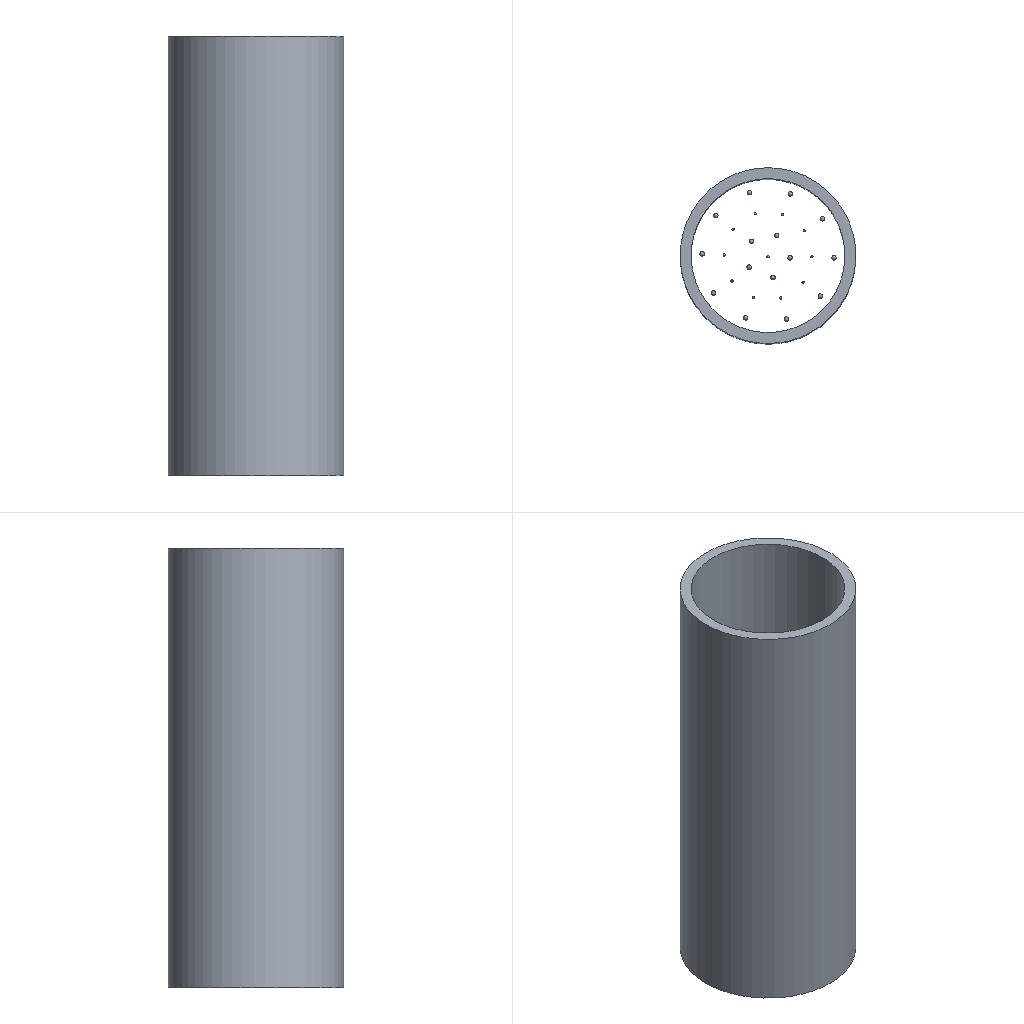Simulation study | abaqus
Set-up summary:
category,name,step,type,value,unit,region
solver,abaqus
solver,version,,,Abaqus/Explicit 2020
units,not stated in the deck,,not stated
analysis,deck,,transient,transient
load_step,Step-1,Step-1,transient
load_step,requested,,,1
mesh,nodes,,,71780
mesh,elements,,,309444
element_type,C3D4,,solid,307524
element_type,C3D8R,,solid,1920
load,load commands in deck,,count,4
bc,support commands in deck,,count,1
material,S,,in results
material,TI,,in results
check,setup vs results,,match,"per instance, exact: element labels, types and connectivity; labels of the nodes the elements use; coordinates of those nodes at SINGLE_PRECISION in 105 of 105 instance(s)"
Abaqus input file, long lists of numbers shortened, first 463 of 1503 lines:
*Heading
** Job name: Job-2 Model name: Model-1-Copy
** Generated by: Abaqus/CAE 2020
*Preprint, echo=NO, model=NO, history=NO, contact=NO
**
** PARTS
**
*Part, name=Part-1
*Node
      1,  -29.793,   -26.691,           0.
      2,  -26.051,  -23.374,           0.
** (3934 more lines like these left out)
*Element, type=C3D8R
   1,   97,   98,  108,  119,    1,    2,   12,   23
   2,  119,  108,  109,  118,   23,   12,   13,   22
** (1918 more lines like these left out)
*Nset, nset=Set-4, generate
    1,  3936,     1
*Elset, elset=Set-4, generate
    1,  1920,     1
** Section: s
*Solid Section, elset=Set-4, material=s
,
*End Part
**
*Part, name=Part-l
*Node
      1,  0.1951,  0.08079,           0.
      2,  0.3827, 0.02388,           0.
** (1007 more lines like these left out)
*Element, type=C3D4
   1,  432,  433,  434,  435
   2,  433,  436,  437,  438
** (4668 more lines like these left out)
*Nset, nset=Set-4, generate
    1,  1009,     1
*Elset, elset=Set-4, generate
    1,  4670,     1
** Section: ti
*Solid Section, elset=Set-4, material=ti
,
*End Part
**
*Part, name=Part-s
*Node
      1,  0.1913, 0.06194,           0.
      2,  0.3536, -0.04645,           0.
** (164 more lines like these left out)
*Element, type=C3D4
  1, 105, 106, 107, 108
  2, 109, 110, 111, 112
** (619 more lines like these left out)
*Nset, nset=Set-4, generate
   1,  166,    1
*Elset, elset=Set-4, generate
   1,  621,    1
** Section: ti
*Solid Section, elset=Set-4, material=ti
,
*End Part
**
**
** ASSEMBLY
**
*Assembly, name=Assembly
**
*Instance, name=Part-1-1, part=Part-1
          0.,           0.,        -150.
*End Instance
**
*Instance, name=Part-l-1, part=Part-l
         30.,           0.,           2.
*End Instance
**
*Instance, name=Part-l-1-rad-2, part=Part-l
24.271, 17.634,           2.
24.271, 17.634,           2., 24.271, 17.634, 3., 36.
*End Instance
**
*Instance, name=Part-l-1-rad-3, part=Part-l
9.271, 28.532,           2.
9.271, 28.532,           2., 9.271, 28.532, 3., 72.
*End Instance
**
*Instance, name=Part-l-1-rad-4, part=Part-l
-9.271, 28.532,           2.
-9.271, 28.532,           2., -9.271, 28.532, 3., 108.
*End Instance
**
*Instance, name=Part-l-1-rad-5, part=Part-l
-24.271, 17.634,           2.
-24.271, 17.634,           2., -24.271, 17.634, 3., 144.
*End Instance
**
*Instance, name=Part-l-1-rad-6, part=Part-l
        -30., 3.67394039744206e-15,           2.
        -30., 3.67394039744206e-15,           2.,         -30., 3.67394039744206e-15,           3.,         180.
*End Instance
**
*Instance, name=Part-l-1-rad-7, part=Part-l
-24.271, -17.634,           2.
-24.271, -17.634,           2., -24.271, -17.634, 3., 216.
*End Instance
**
*Instance, name=Part-l-1-rad-8, part=Part-l
-9.271, -28.532,           2.
-9.271, -28.532,           2., -9.271, -28.532, 1., 108.
*End Instance
**
*Instance, name=Part-l-1-rad-9, part=Part-l
9.271, -28.532,           2.
9.271, -28.532,           2., 9.271, -28.532, 1., 72.
*End Instance
**
*Instance, name=Part-l-1-rad-10, part=Part-l
24.271, -17.634,           2.
24.271, -17.634,           2., 24.271, -17.634, 1., 36.
*End Instance
**
*Instance, name=Part-s-1, part=Part-s
         20.,           0.,          1.5
*End Instance
**
*Instance, name=Part-s-1-rad-2, part=Part-s
16.18, 11.756,          1.5
16.18, 11.756,          1.5, 16.18, 11.756, 2.5, 36.
*End Instance
**
*Instance, name=Part-s-1-rad-3, part=Part-s
6.18, 19.021,          1.5
6.18, 19.021,          1.5, 6.18, 19.021, 2.5, 72.
*End Instance
**
*Instance, name=Part-s-1-rad-4, part=Part-s
-6.18, 19.021,          1.5
-6.18, 19.021,          1.5, -6.18, 19.021, 2.5, 108.
*End Instance
**
*Instance, name=Part-s-1-rad-5, part=Part-s
-16.18, 11.756,          1.5
-16.18, 11.756,          1.5, -16.18, 11.756, 2.5, 144.
*End Instance
**
*Instance, name=Part-s-1-rad-6, part=Part-s
        -20., 2.44929359829471e-15,          1.5
        -20., 2.44929359829471e-15,          1.5,         -20., 2.44929359829471e-15,          2.5,         180.
*End Instance
**
*Instance, name=Part-s-1-rad-7, part=Part-s
-16.18, -11.756,          1.5
-16.18, -11.756,          1.5, -16.18, -11.756, 2.5, 216.
*End Instance
**
*Instance, name=Part-s-1-rad-8, part=Part-s
-6.18, -19.021,          1.5
-6.18, -19.021,          1.5, -6.18, -19.021, 0.5, 108.
*End Instance
**
*Instance, name=Part-s-1-rad-9, part=Part-s
6.18, -19.021,          1.5
6.18, -19.021,          1.5, 6.18, -19.021, 0.5, 72.
*End Instance
**
*Instance, name=Part-s-1-rad-10, part=Part-s
16.18, -11.756,          1.5
16.18, -11.756,          1.5, 16.18, -11.756, 0.5, 36.
*End Instance
**
*Instance, name=Part-l-2, part=Part-l
         10.,           0.,           2.
*End Instance
**
*Instance, name=Part-l-2-rad-2, part=Part-l
3.09, 9.511,           2.
3.09, 9.511,           2., 3.09, 9.511, 3., 72.
*End Instance
**
*Instance, name=Part-l-2-rad-3, part=Part-l
-8.09, 5.878,           2.
-8.09, 5.878,           2., -8.09, 5.878, 3., 144.
*End Instance
**
*Instance, name=Part-l-2-rad-4, part=Part-l
-8.09, -5.878,           2.
-8.09, -5.878,           2., -8.09, -5.878, 3., 216.
*End Instance
**
*Instance, name=Part-l-2-rad-5, part=Part-l
3.09, -9.511,           2.
3.09, -9.511,           2., 3.09, -9.511, 1., 72.
*End Instance
**
*Instance, name=Part-s-2, part=Part-s
          0.,           0.,          1.5
*End Instance
**
*Instance, name=Part-l-1-lin-2-1, part=Part-l
         30.,           0.,         -13.
*End Instance
**
*Instance, name=Part-l-1-lin-3-1, part=Part-l
         30.,           0.,         -28.
*End Instance
**
*Instance, name=Part-l-1-lin-4-1, part=Part-l
         30.,           0.,         -43.
*End Instance
**
*Instance, name=Part-l-1-rad-2-lin-2-1, part=Part-l
24.271, 17.634,         -13.
24.271, 17.634,         -13., 24.271, 17.634, -12., 36.
*End Instance
**
*Instance, name=Part-l-1-rad-2-lin-3-1, part=Part-l
24.271, 17.634,         -28.
24.271, 17.634,         -28., 24.271, 17.634, -27., 36.
*End Instance
**
*Instance, name=Part-l-1-rad-2-lin-4-1, part=Part-l
24.271, 17.634,         -43.
24.271, 17.634,         -43., 24.271, 17.634, -42., 36.
*End Instance
**
*Instance, name=Part-l-1-rad-4-lin-2-1, part=Part-l
-9.271, 28.532,         -13.
-9.271, 28.532,         -13., -9.271, 28.532, -12., 108.
*End Instance
**
*Instance, name=Part-l-1-rad-4-lin-3-1, part=Part-l
-9.271, 28.532,         -28.
-9.271, 28.532,         -28., -9.271, 28.532, -27., 108.
*End Instance
**
*Instance, name=Part-l-1-rad-4-lin-4-1, part=Part-l
-9.271, 28.532,         -43.
-9.271, 28.532,         -43., -9.271, 28.532, -42., 108.
*End Instance
**
*Instance, name=Part-l-1-rad-6-lin-2-1, part=Part-l
        -30., 3.67394039744206e-15,         -13.
        -30., 3.67394039744206e-15,         -13.,         -30., 3.67394039744206e-15,         -12.,         180.
*End Instance
**
*Instance, name=Part-l-1-rad-6-lin-3-1, part=Part-l
        -30., 3.67394039744206e-15,         -28.
        -30., 3.67394039744206e-15,         -28.,         -30., 3.67394039744206e-15,         -27.,         180.
*End Instance
**
*Instance, name=Part-l-1-rad-6-lin-4-1, part=Part-l
        -30., 3.67394039744206e-15,         -43.
        -30., 3.67394039744206e-15,         -43.,         -30., 3.67394039744206e-15,         -42.,         180.
*End Instance
**
*Instance, name=Part-l-1-rad-8-lin-2-1, part=Part-l
-9.271, -28.532,         -13.
-9.271, -28.532,         -13., -9.271, -28.532, -14., 108.
*End Instance
**
*Instance, name=Part-l-1-rad-8-lin-3-1, part=Part-l
-9.271, -28.532,         -28.
-9.271, -28.532,         -28., -9.271, -28.532, -29., 108.
*End Instance
**
*Instance, name=Part-l-1-rad-8-lin-4-1, part=Part-l
-9.271, -28.532,         -43.
-9.271, -28.532,         -43., -9.271, -28.532, -44., 108.
*End Instance
**
*Instance, name=Part-l-1-rad-10-lin-2-1, part=Part-l
24.271, -17.634,         -13.
24.271, -17.634,         -13., 24.271, -17.634, -14., 36.
*End Instance
**
*Instance, name=Part-l-1-rad-10-lin-3-1, part=Part-l
24.271, -17.634,         -28.
24.271, -17.634,         -28., 24.271, -17.634, -29., 36.
*End Instance
**
*Instance, name=Part-l-1-rad-10-lin-4-1, part=Part-l
24.271, -17.634,         -43.
24.271, -17.634,         -43., 24.271, -17.634, -44., 36.
*End Instance
**
*Instance, name=Part-s-1-rad-2-lin-2-1, part=Part-s
16.18, 11.756,        -13.5
16.18, 11.756,        -13.5, 16.18, 11.756, -12.5, 36.
*End Instance
**
*Instance, name=Part-s-1-rad-2-lin-3-1, part=Part-s
16.18, 11.756,        -28.5
16.18, 11.756,        -28.5, 16.18, 11.756, -27.5, 36.
*End Instance
**
*Instance, name=Part-s-1-rad-2-lin-4-1, part=Part-s
16.18, 11.756,        -43.5
16.18, 11.756,        -43.5, 16.18, 11.756, -42.5, 36.
*End Instance
**
*Instance, name=Part-s-1-rad-4-lin-2-1, part=Part-s
-6.18, 19.021,        -13.5
-6.18, 19.021,        -13.5, -6.18, 19.021, -12.5, 108.
*End Instance
**
*Instance, name=Part-s-1-rad-4-lin-3-1, part=Part-s
-6.18, 19.021,        -28.5
-6.18, 19.021,        -28.5, -6.18, 19.021, -27.5, 108.
*End Instance
**
*Instance, name=Part-s-1-rad-4-lin-4-1, part=Part-s
-6.18, 19.021,        -43.5
-6.18, 19.021,        -43.5, -6.18, 19.021, -42.5, 108.
*End Instance
**
*Instance, name=Part-s-1-rad-6-lin-2-1, part=Part-s
        -20., 2.44929359829471e-15,        -13.5
        -20., 2.44929359829471e-15,        -13.5,         -20., 2.44929359829471e-15,        -12.5,         180.
*End Instance
**
*Instance, name=Part-s-1-rad-6-lin-3-1, part=Part-s
        -20., 2.44929359829471e-15,        -28.5
        -20., 2.44929359829471e-15,        -28.5,         -20., 2.44929359829471e-15,        -27.5,         180.
*End Instance
**
*Instance, name=Part-s-1-rad-6-lin-4-1, part=Part-s
        -20., 2.44929359829471e-15,        -43.5
        -20., 2.44929359829471e-15,        -43.5,         -20., 2.44929359829471e-15,        -42.5,         180.
*End Instance
**
*Instance, name=Part-s-1-rad-8-lin-2-1, part=Part-s
-6.18, -19.021,        -13.5
-6.18, -19.021,        -13.5, -6.18, -19.021, -14.5, 108.
*End Instance
**
*Instance, name=Part-s-1-rad-8-lin-3-1, part=Part-s
-6.18, -19.021,        -28.5
-6.18, -19.021,        -28.5, -6.18, -19.021, -29.5, 108.
*End Instance
**
*Instance, name=Part-s-1-rad-8-lin-4-1, part=Part-s
-6.18, -19.021,        -43.5
-6.18, -19.021,        -43.5, -6.18, -19.021, -44.5, 108.
*End Instance
**
*Instance, name=Part-l-2-lin-2-1, part=Part-l
         10.,           0.,         -13.
*End Instance
**
*Instance, name=Part-l-2-lin-3-1, part=Part-l
         10.,           0.,         -28.
*End Instance
**
*Instance, name=Part-l-2-lin-4-1, part=Part-l
         10.,           0.,         -43.
*End Instance
**
*Instance, name=Part-l-2-rad-2-lin-2-1, part=Part-l
3.09, 9.511,         -13.
3.09, 9.511,         -13., 3.09, 9.511, -12., 72.
*End Instance
**
*Instance, name=Part-l-2-rad-2-lin-3-1, part=Part-l
3.09, 9.511,         -28.
3.09, 9.511,         -28., 3.09, 9.511, -27., 72.
*End Instance
**
*Instance, name=Part-l-2-rad-2-lin-4-1, part=Part-l
3.09, 9.511,         -43.
3.09, 9.511,         -43., 3.09, 9.511, -42., 72.
*End Instance
**
*Instance, name=Part-l-2-rad-4-lin-2-1, part=Part-l
-8.09, -5.878,         -13.
-8.09, -5.878,         -13., -8.09, -5.878, -12., 216.
*End Instance
**
*Instance, name=Part-l-2-rad-4-lin-3-1, part=Part-l
-8.09, -5.878,         -28.
-8.09, -5.878,         -28., -8.09, -5.878, -27., 216.
*End Instance
**
*Instance, name=Part-l-2-rad-4-lin-4-1, part=Part-l
-8.09, -5.878,         -43.
-8.09, -5.878,         -43., -8.09, -5.878, -42., 216.
*End Instance
**
*Instance, name=Part-s-1-rad-10-lin-2-1, part=Part-s
16.18, -11.756,        -13.5
16.18, -11.756,        -13.5, 16.18, -11.756, -14.5, 36.
*End Instance
**
*Instance, name=Part-s-1-rad-10-lin-3-1, part=Part-s
16.18, -11.756,        -28.5
16.18, -11.756,        -28.5, 16.18, -11.756, -29.5, 36.
*End Instance
**
*Instance, name=Part-s-1-rad-10-lin-4-1, part=Part-s
16.18, -11.756,        -43.5
16.18, -11.756,        -43.5, 16.18, -11.756, -44.5, 36.
*End Instance
**
*Instance, name=Part-s-2-lin-2-1, part=Part-s
          0.,           0.,        -13.5
*End Instance
**
*Instance, name=Part-s-2-lin-3-1, part=Part-s
          0.,           0.,        -28.5
*End Instance
**
*Instance, name=Part-s-2-lin-4-1, part=Part-s
          0.,           0.,        -43.5
*End Instance
**
*Instance, name=Part-l-1-rad-3-lin-2-1, part=Part-l
9.271, 28.532,         -13.
9.271, 28.532,         -13., 9.271, 28.532, -12., 72.
*End Instance
**
*Instance, name=Part-l-1-rad-3-lin-3-1, part=Part-l
9.271, 28.532,         -28.
9.271, 28.532,         -28., 9.271, 28.532, -27., 72.
*End Instance
**
*Instance, name=Part-l-1-rad-3-lin-4-1, part=Part-l
9.271, 28.532,         -43.
9.271, 28.532,         -43., 9.271, 28.532, -42., 72.
*End Instance
**
*Instance, name=Part-l-1-rad-5-lin-2-1, part=Part-l
-24.271, 17.634,         -13.
-24.271, 17.634,         -13., -24.271, 17.634, -12., 144.
*End Instance
**
*Instance, name=Part-l-1-rad-5-lin-3-1, part=Part-l
-24.271, 17.634,         -28.
-24.271, 17.634,         -28., -24.271, 17.634, -27., 144.
*End Instance
**
*Instance, name=Part-l-1-rad-5-lin-4-1, part=Part-l
-24.271, 17.634,         -43.
-24.271, 17.634,         -43., -24.271, 17.634, -42., 144.
*End Instance
**
*Instance, name=Part-l-1-rad-7-lin-2-1, part=Part-l
-24.271, -17.634,         -13.
-24.271, -17.634,         -13., -24.271, -17.634, -12., 216.
*End Instance
**
*Instance, name=Part-l-1-rad-7-lin-3-1, part=Part-l
-24.271, -17.634,         -28.
-24.271, -17.634,         -28., -24.271, -17.634, -27., 216.
*End Instance
**
*Instance, name=Part-l-1-rad-7-lin-4-1, part=Part-l
-24.271, -17.634,         -43.
-24.271, -17.634,         -43., -24.271, -17.634, -42., 216.
*End Instance
**
*Instance, name=Part-l-1-rad-9-lin-2-1, part=Part-l
9.271, -28.532,         -13.
9.271, -28.532,         -13., 9.271, -28.532, -14., 72.
*End Instance
**
*Instance, name=Part-l-1-rad-9-lin-3-1, part=Part-l
Last 582 lines:
    1,  1009,     1
*Nset, nset=Set-7, instance=Part-s-1-rad-4-lin-3-1, generate
   1,  166,    1
*Nset, nset=Set-7, instance=Part-l-2-rad-2-lin-3-1, generate
    1,  1009,     1
*Nset, nset=Set-7, instance=Part-s-1-rad-3-lin-3-1, generate
   1,  166,    1
*Nset, nset=Set-7, instance=Part-l-1-rad-3-lin-3-1, generate
    1,  1009,     1
*Nset, nset=Set-7, instance=Part-l-2-rad-3-lin-3-1, generate
    1,  1009,     1
*Nset, nset=Set-7, instance=Part-l-1-rad-10-lin-3-1, generate
    1,  1009,     1
*Nset, nset=Set-7, instance=Part-s-1-rad-8-lin-3-1, generate
   1,  166,    1
*Nset, nset=Set-7, instance=Part-s-1-lin-3-1, generate
   1,  166,    1
*Nset, nset=Set-7, instance=Part-l-1-rad-7-lin-3-1, generate
    1,  1009,     1
*Nset, nset=Set-7, instance=Part-s-1-rad-10-lin-3-1, generate
   1,  166,    1
*Nset, nset=Set-7, instance=Part-s-1-rad-7-lin-3-1, generate
   1,  166,    1
*Elset, elset=Set-7, instance=Part-l-1-lin-3-1, generate
    1,  4670,     1
*Elset, elset=Set-7, instance=Part-l-1-rad-2-lin-3-1, generate
    1,  4670,     1
*Elset, elset=Set-7, instance=Part-l-1-rad-4-lin-3-1, generate
    1,  4670,     1
*Elset, elset=Set-7, instance=Part-l-1-rad-8-lin-3-1, generate
    1,  4670,     1
*Elset, elset=Set-7, instance=Part-s-1-rad-6-lin-3-1, generate
   1,  621,    1
*Elset, elset=Set-7, instance=Part-l-2-rad-5-lin-3-1, generate
    1,  4670,     1
*Elset, elset=Set-7, instance=Part-l-1-rad-5-lin-3-1, generate
    1,  4670,     1
*Elset, elset=Set-7, instance=Part-l-2-rad-4-lin-3-1, generate
    1,  4670,     1
*Elset, elset=Set-7, instance=Part-s-1-rad-5-lin-3-1, generate
   1,  621,    1
*Elset, elset=Set-7, instance=Part-s-1-rad-2-lin-3-1, generate
   1,  621,    1
*Elset, elset=Set-7, instance=Part-s-2-lin-3-1, generate
   1,  621,    1
*Elset, elset=Set-7, instance=Part-s-1-rad-9-lin-3-1, generate
   1,  621,    1
*Elset, elset=Set-7, instance=Part-l-2-lin-3-1, generate
    1,  4670,     1
*Elset, elset=Set-7, instance=Part-l-1-rad-9-lin-3-1, generate
    1,  4670,     1
*Elset, elset=Set-7, instance=Part-l-1-rad-6-lin-3-1, generate
    1,  4670,     1
*Elset, elset=Set-7, instance=Part-s-1-rad-4-lin-3-1, generate
   1,  621,    1
*Elset, elset=Set-7, instance=Part-l-2-rad-2-lin-3-1, generate
    1,  4670,     1
*Elset, elset=Set-7, instance=Part-s-1-rad-3-lin-3-1, generate
   1,  621,    1
*Elset, elset=Set-7, instance=Part-l-1-rad-3-lin-3-1, generate
    1,  4670,     1
*Elset, elset=Set-7, instance=Part-l-2-rad-3-lin-3-1, generate
    1,  4670,     1
*Elset, elset=Set-7, instance=Part-l-1-rad-10-lin-3-1, generate
    1,  4670,     1
*Elset, elset=Set-7, instance=Part-s-1-rad-8-lin-3-1, generate
   1,  621,    1
*Elset, elset=Set-7, instance=Part-s-1-lin-3-1, generate
   1,  621,    1
*Elset, elset=Set-7, instance=Part-l-1-rad-7-lin-3-1, generate
    1,  4670,     1
*Elset, elset=Set-7, instance=Part-s-1-rad-10-lin-3-1, generate
   1,  621,    1
*Elset, elset=Set-7, instance=Part-s-1-rad-7-lin-3-1, generate
   1,  621,    1
*Nset, nset=Set-8, instance=Part-l-1-lin-4-1, generate
    1,  1009,     1
*Nset, nset=Set-8, instance=Part-l-1-rad-2-lin-4-1, generate
    1,  1009,     1
*Nset, nset=Set-8, instance=Part-l-1-rad-6-lin-4-1, generate
    1,  1009,     1
*Nset, nset=Set-8, instance=Part-l-1-rad-10-lin-4-1, generate
    1,  1009,     1
*Nset, nset=Set-8, instance=Part-s-1-rad-10-lin-4-1, generate
   1,  166,    1
*Nset, nset=Set-8, instance=Part-s-1-rad-7-lin-4-1, generate
   1,  166,    1
*Nset, nset=Set-8, instance=Part-s-1-rad-8-lin-4-1, generate
   1,  166,    1
*Nset, nset=Set-8, instance=Part-s-1-lin-4-1, generate
   1,  166,    1
*Nset, nset=Set-8, instance=Part-l-1-rad-7-lin-4-1, generate
    1,  1009,     1
*Nset, nset=Set-8, instance=Part-s-1-rad-4-lin-4-1, generate
   1,  166,    1
*Nset, nset=Set-8, instance=Part-l-2-rad-2-lin-4-1, generate
    1,  1009,     1
*Nset, nset=Set-8, instance=Part-s-1-rad-3-lin-4-1, generate
   1,  166,    1
*Nset, nset=Set-8, instance=Part-l-1-rad-3-lin-4-1, generate
    1,  1009,     1
*Nset, nset=Set-8, instance=Part-l-2-rad-3-lin-4-1, generate
    1,  1009,     1
*Nset, nset=Set-8, instance=Part-l-1-rad-4-lin-4-1, generate
    1,  1009,     1
*Nset, nset=Set-8, instance=Part-l-1-rad-8-lin-4-1, generate
    1,  1009,     1
*Nset, nset=Set-8, instance=Part-s-1-rad-6-lin-4-1, generate
   1,  166,    1
*Nset, nset=Set-8, instance=Part-l-2-rad-5-lin-4-1, generate
    1,  1009,     1
*Nset, nset=Set-8, instance=Part-l-1-rad-5-lin-4-1, generate
    1,  1009,     1
*Nset, nset=Set-8, instance=Part-l-2-rad-4-lin-4-1, generate
    1,  1009,     1
*Nset, nset=Set-8, instance=Part-s-1-rad-5-lin-4-1, generate
   1,  166,    1
*Nset, nset=Set-8, instance=Part-s-1-rad-2-lin-4-1, generate
   1,  166,    1
*Nset, nset=Set-8, instance=Part-s-2-lin-4-1, generate
   1,  166,    1
*Nset, nset=Set-8, instance=Part-s-1-rad-9-lin-4-1, generate
   1,  166,    1
*Nset, nset=Set-8, instance=Part-l-2-lin-4-1, generate
    1,  1009,     1
*Nset, nset=Set-8, instance=Part-l-1-rad-9-lin-4-1, generate
    1,  1009,     1
*Elset, elset=Set-8, instance=Part-l-1-lin-4-1, generate
    1,  4670,     1
*Elset, elset=Set-8, instance=Part-l-1-rad-2-lin-4-1, generate
    1,  4670,     1
*Elset, elset=Set-8, instance=Part-l-1-rad-6-lin-4-1, generate
    1,  4670,     1
*Elset, elset=Set-8, instance=Part-l-1-rad-10-lin-4-1, generate
    1,  4670,     1
*Elset, elset=Set-8, instance=Part-s-1-rad-10-lin-4-1, generate
   1,  621,    1
*Elset, elset=Set-8, instance=Part-s-1-rad-7-lin-4-1, generate
   1,  621,    1
*Elset, elset=Set-8, instance=Part-s-1-rad-8-lin-4-1, generate
   1,  621,    1
*Elset, elset=Set-8, instance=Part-s-1-lin-4-1, generate
   1,  621,    1
*Elset, elset=Set-8, instance=Part-l-1-rad-7-lin-4-1, generate
    1,  4670,     1
*Elset, elset=Set-8, instance=Part-s-1-rad-4-lin-4-1, generate
   1,  621,    1
*Elset, elset=Set-8, instance=Part-l-2-rad-2-lin-4-1, generate
    1,  4670,     1
*Elset, elset=Set-8, instance=Part-s-1-rad-3-lin-4-1, generate
   1,  621,    1
*Elset, elset=Set-8, instance=Part-l-1-rad-3-lin-4-1, generate
    1,  4670,     1
*Elset, elset=Set-8, instance=Part-l-2-rad-3-lin-4-1, generate
    1,  4670,     1
*Elset, elset=Set-8, instance=Part-l-1-rad-4-lin-4-1, generate
    1,  4670,     1
*Elset, elset=Set-8, instance=Part-l-1-rad-8-lin-4-1, generate
    1,  4670,     1
*Elset, elset=Set-8, instance=Part-s-1-rad-6-lin-4-1, generate
   1,  621,    1
*Elset, elset=Set-8, instance=Part-l-2-rad-5-lin-4-1, generate
    1,  4670,     1
*Elset, elset=Set-8, instance=Part-l-1-rad-5-lin-4-1, generate
    1,  4670,     1
*Elset, elset=Set-8, instance=Part-l-2-rad-4-lin-4-1, generate
    1,  4670,     1
*Elset, elset=Set-8, instance=Part-s-1-rad-5-lin-4-1, generate
   1,  621,    1
*Elset, elset=Set-8, instance=Part-s-1-rad-2-lin-4-1, generate
   1,  621,    1
*Elset, elset=Set-8, instance=Part-s-2-lin-4-1, generate
   1,  621,    1
*Elset, elset=Set-8, instance=Part-s-1-rad-9-lin-4-1, generate
   1,  621,    1
*Elset, elset=Set-8, instance=Part-l-2-lin-4-1, generate
    1,  4670,     1
*Elset, elset=Set-8, instance=Part-l-1-rad-9-lin-4-1, generate
    1,  4670,     1
*Elset, elset=_s_Surf-2_S3, internal, instance=Part-l-1
   30,   47,   54,   77,   80,  114,  145,  165,  199,  207,  217,  244,  259,  357,  363,  400
  418,  419,  462,  482,  501,  525,  526,  546,  597,  610,  640,  656,  662,  671,  692,  712
** (47 more lines like these left out)
*Elset, elset=_s_Surf-2_S3, internal, instance=Part-l-1-rad-2
   30,   47,   54,   77,   80,  114,  145,  165,  199,  207,  217,  244,  259,  357,  363,  400
  418,  419,  462,  482,  501,  525,  526,  546,  597,  610,  640,  656,  662,  671,  692,  712
** (47 more lines like these left out)
*Elset, elset=_s_Surf-2_S3, internal, instance=Part-l-1-rad-3
   30,   47,   54,   77,   80,  114,  145,  165,  199,  207,  217,  244,  259,  357,  363,  400
  418,  419,  462,  482,  501,  525,  526,  546,  597,  610,  640,  656,  662,  671,  692,  712
** (47 more lines like these left out)
*Elset, elset=_s_Surf-2_S3, internal, instance=Part-l-1-rad-5
   30,   47,   54,   77,   80,  114,  145,  165,  199,  207,  217,  244,  259,  357,  363,  400
  418,  419,  462,  482,  501,  525,  526,  546,  597,  610,  640,  656,  662,  671,  692,  712
** (47 more lines like these left out)
*Elset, elset=_s_Surf-2_S3, internal, instance=Part-s-1-rad-3
   7,  13,  19,  28,  38,  42,  98, 107, 112, 119, 138, 158, 161, 170, 177, 178
 188, 195, 199, 213, 231, 244, 249, 255, 263, 289, 292, 310, 326, 329, 344, 371
** (10 more lines like these left out)
*Elset, elset=_s_Surf-2_S3, internal, instance=Part-l-2
   30,   47,   54,   77,   80,  114,  145,  165,  199,  207,  217,  244,  259,  357,  363,  400
  418,  419,  462,  482,  501,  525,  526,  546,  597,  610,  640,  656,  662,  671,  692,  712
** (47 more lines like these left out)
*Elset, elset=_s_Surf-2_S3, internal, instance=Part-l-1-rad-9
   30,   47,   54,   77,   80,  114,  145,  165,  199,  207,  217,  244,  259,  357,  363,  400
  418,  419,  462,  482,  501,  525,  526,  546,  597,  610,  640,  656,  662,  671,  692,  712
** (47 more lines like these left out)
*Elset, elset=_s_Surf-2_S3, internal, instance=Part-s-1-rad-7
   7,  13,  19,  28,  38,  42,  98, 107, 112, 119, 138, 158, 161, 170, 177, 178
 188, 195, 199, 213, 231, 244, 249, 255, 263, 289, 292, 310, 326, 329, 344, 371
** (10 more lines like these left out)
*Elset, elset=_s_Surf-2_S3, internal, instance=Part-l-2-rad-5
   30,   47,   54,   77,   80,  114,  145,  165,  199,  207,  217,  244,  259,  357,  363,  400
  418,  419,  462,  482,  501,  525,  526,  546,  597,  610,  640,  656,  662,  671,  692,  712
** (47 more lines like these left out)
*Elset, elset=_s_Surf-2_S3, internal, instance=Part-l-1-rad-7
   30,   47,   54,   77,   80,  114,  145,  165,  199,  207,  217,  244,  259,  357,  363,  400
  418,  419,  462,  482,  501,  525,  526,  546,  597,  610,  640,  656,  662,  671,  692,  712
** (47 more lines like these left out)
*Elset, elset=_s_Surf-2_S3, internal, instance=Part-s-1-rad-5
   7,  13,  19,  28,  38,  42,  98, 107, 112, 119, 138, 158, 161, 170, 177, 178
 188, 195, 199, 213, 231, 244, 249, 255, 263, 289, 292, 310, 326, 329, 344, 371
** (10 more lines like these left out)
*Elset, elset=_s_Surf-2_S3, internal, instance=Part-l-2-rad-3
   30,   47,   54,   77,   80,  114,  145,  165,  199,  207,  217,  244,  259,  357,  363,  400
  418,  419,  462,  482,  501,  525,  526,  546,  597,  610,  640,  656,  662,  671,  692,  712
** (47 more lines like these left out)
*Elset, elset=_s_Surf-2_S3, internal, instance=Part-s-1
   7,  13,  19,  28,  38,  42,  98, 107, 112, 119, 138, 158, 161, 170, 177, 178
 188, 195, 199, 213, 231, 244, 249, 255, 263, 289, 292, 310, 326, 329, 344, 371
** (10 more lines like these left out)
*Elset, elset=_s_Surf-2_S3, internal, instance=Part-s-1-rad-9
   7,  13,  19,  28,  38,  42,  98, 107, 112, 119, 138, 158, 161, 170, 177, 178
 188, 195, 199, 213, 231, 244, 249, 255, 263, 289, 292, 310, 326, 329, 344, 371
** (10 more lines like these left out)
*Elset, elset=_s_Surf-2_S3, internal, instance=Part-l-1-rad-4
   30,   47,   54,   77,   80,  114,  145,  165,  199,  207,  217,  244,  259,  357,  363,  400
  418,  419,  462,  482,  501,  525,  526,  546,  597,  610,  640,  656,  662,  671,  692,  712
** (47 more lines like these left out)
*Elset, elset=_s_Surf-2_S3, internal, instance=Part-l-1-rad-6
   30,   47,   54,   77,   80,  114,  145,  165,  199,  207,  217,  244,  259,  357,  363,  400
  418,  419,  462,  482,  501,  525,  526,  546,  597,  610,  640,  656,  662,  671,  692,  712
** (47 more lines like these left out)
*Elset, elset=_s_Surf-2_S3, internal, instance=Part-s-1-rad-4
   7,  13,  19,  28,  38,  42,  98, 107, 112, 119, 138, 158, 161, 170, 177, 178
 188, 195, 199, 213, 231, 244, 249, 255, 263, 289, 292, 310, 326, 329, 344, 371
** (10 more lines like these left out)
*Elset, elset=_s_Surf-2_S3, internal, instance=Part-l-2-rad-2
   30,   47,   54,   77,   80,  114,  145,  165,  199,  207,  217,  244,  259,  357,  363,  400
  418,  419,  462,  482,  501,  525,  526,  546,  597,  610,  640,  656,  662,  671,  692,  712
** (47 more lines like these left out)
*Elset, elset=_s_Surf-2_S3, internal, instance=Part-l-1-rad-10
   30,   47,   54,   77,   80,  114,  145,  165,  199,  207,  217,  244,  259,  357,  363,  400
  418,  419,  462,  482,  501,  525,  526,  546,  597,  610,  640,  656,  662,  671,  692,  712
** (47 more lines like these left out)
*Elset, elset=_s_Surf-2_S3, internal, instance=Part-s-1-rad-8
   7,  13,  19,  28,  38,  42,  98, 107, 112, 119, 138, 158, 161, 170, 177, 178
 188, 195, 199, 213, 231, 244, 249, 255, 263, 289, 292, 310, 326, 329, 344, 371
** (10 more lines like these left out)
*Elset, elset=_s_Surf-2_S3, internal, instance=Part-s-2
   7,  13,  19,  28,  38,  42,  98, 107, 112, 119, 138, 158, 161, 170, 177, 178
 188, 195, 199, 213, 231, 244, 249, 255, 263, 289, 292, 310, 326, 329, 344, 371
** (10 more lines like these left out)
*Elset, elset=_s_Surf-2_S3, internal, instance=Part-l-1-rad-8
   30,   47,   54,   77,   80,  114,  145,  165,  199,  207,  217,  244,  259,  357,  363,  400
  418,  419,  462,  482,  501,  525,  526,  546,  597,  610,  640,  656,  662,  671,  692,  712
** (47 more lines like these left out)
*Elset, elset=_s_Surf-2_S3, internal, instance=Part-s-1-rad-6
   7,  13,  19,  28,  38,  42,  98, 107, 112, 119, 138, 158, 161, 170, 177, 178
 188, 195, 199, 213, 231, 244, 249, 255, 263, 289, 292, 310, 326, 329, 344, 371
** (10 more lines like these left out)
*Elset, elset=_s_Surf-2_S3, internal, instance=Part-l-2-rad-4
   30,   47,   54,   77,   80,  114,  145,  165,  199,  207,  217,  244,  259,  357,  363,  400
  418,  419,  462,  482,  501,  525,  526,  546,  597,  610,  640,  656,  662,  671,  692,  712
** (47 more lines like these left out)
*Elset, elset=_s_Surf-2_S3, internal, instance=Part-s-1-rad-2
   7,  13,  19,  28,  38,  42,  98, 107, 112, 119, 138, 158, 161, 170, 177, 178
 188, 195, 199, 213, 231, 244, 249, 255, 263, 289, 292, 310, 326, 329, 344, 371
** (10 more lines like these left out)
*Elset, elset=_s_Surf-2_S3, internal, instance=Part-s-1-rad-10
   7,  13,  19,  28,  38,  42,  98, 107, 112, 119, 138, 158, 161, 170, 177, 178
 188, 195, 199, 213, 231, 244, 249, 255, 263, 289, 292, 310, 326, 329, 344, 371
** (10 more lines like these left out)
*Elset, elset=_s_Surf-2_S4, internal, instance=Part-l-1
   92,  253,  267,  774,  957, 1766, 1772, 2198, 2474, 2492, 2589, 2776, 2788, 2789, 2811, 2934
 3094, 3208, 3334, 3386, 3404, 3412, 3566, 3733, 3836, 3843, 3934, 4003, 4024, 4073, 4096, 4179
** (1 more lines like these left out)
*Elset, elset=_s_Surf-2_S4, internal, instance=Part-l-1-rad-2
   92,  253,  267,  774,  957, 1766, 1772, 2198, 2474, 2492, 2589, 2776, 2788, 2789, 2811, 2934
 3094, 3208, 3334, 3386, 3404, 3412, 3566, 3733, 3836, 3843, 3934, 4003, 4024, 4073, 4096, 4179
** (1 more lines like these left out)
*Elset, elset=_s_Surf-2_S4, internal, instance=Part-l-1-rad-3
   92,  253,  267,  774,  957, 1766, 1772, 2198, 2474, 2492, 2589, 2776, 2788, 2789, 2811, 2934
 3094, 3208, 3334, 3386, 3404, 3412, 3566, 3733, 3836, 3843, 3934, 4003, 4024, 4073, 4096, 4179
** (1 more lines like these left out)
*Elset, elset=_s_Surf-2_S4, internal, instance=Part-l-1-rad-5
   92,  253,  267,  774,  957, 1766, 1772, 2198, 2474, 2492, 2589, 2776, 2788, 2789, 2811, 2934
 3094, 3208, 3334, 3386, 3404, 3412, 3566, 3733, 3836, 3843, 3934, 4003, 4024, 4073, 4096, 4179
** (1 more lines like these left out)
*Elset, elset=_s_Surf-2_S4, internal, instance=Part-s-1-rad-3
  40,  94, 202, 219, 438, 444, 481, 513, 610
*Elset, elset=_s_Surf-2_S4, internal, instance=Part-l-2
   92,  253,  267,  774,  957, 1766, 1772, 2198, 2474, 2492, 2589, 2776, 2788, 2789, 2811, 2934
 3094, 3208, 3334, 3386, 3404, 3412, 3566, 3733, 3836, 3843, 3934, 4003, 4024, 4073, 4096, 4179
** (1 more lines like these left out)
*Elset, elset=_s_Surf-2_S4, internal, instance=Part-l-1-rad-9
   92,  253,  267,  774,  957, 1766, 1772, 2198, 2474, 2492, 2589, 2776, 2788, 2789, 2811, 2934
 3094, 3208, 3334, 3386, 3404, 3412, 3566, 3733, 3836, 3843, 3934, 4003, 4024, 4073, 4096, 4179
** (1 more lines like these left out)
*Elset, elset=_s_Surf-2_S4, internal, instance=Part-s-1-rad-7
  40,  94, 202, 219, 438, 444, 481, 513, 610
*Elset, elset=_s_Surf-2_S4, internal, instance=Part-l-2-rad-5
   92,  253,  267,  774,  957, 1766, 1772, 2198, 2474, 2492, 2589, 2776, 2788, 2789, 2811, 2934
 3094, 3208, 3334, 3386, 3404, 3412, 3566, 3733, 3836, 3843, 3934, 4003, 4024, 4073, 4096, 4179
** (1 more lines like these left out)
*Elset, elset=_s_Surf-2_S4, internal, instance=Part-l-1-rad-7
   92,  253,  267,  774,  957, 1766, 1772, 2198, 2474, 2492, 2589, 2776, 2788, 2789, 2811, 2934
 3094, 3208, 3334, 3386, 3404, 3412, 3566, 3733, 3836, 3843, 3934, 4003, 4024, 4073, 4096, 4179
** (1 more lines like these left out)
*Elset, elset=_s_Surf-2_S4, internal, instance=Part-s-1-rad-5
  40,  94, 202, 219, 438, 444, 481, 513, 610
*Elset, elset=_s_Surf-2_S4, internal, instance=Part-l-2-rad-3
   92,  253,  267,  774,  957, 1766, 1772, 2198, 2474, 2492, 2589, 2776, 2788, 2789, 2811, 2934
 3094, 3208, 3334, 3386, 3404, 3412, 3566, 3733, 3836, 3843, 3934, 4003, 4024, 4073, 4096, 4179
** (1 more lines like these left out)
*Elset, elset=_s_Surf-2_S4, internal, instance=Part-s-1
  40,  94, 202, 219, 438, 444, 481, 513, 610
*Elset, elset=_s_Surf-2_S4, internal, instance=Part-s-1-rad-9
  40,  94, 202, 219, 438, 444, 481, 513, 610
*Elset, elset=_s_Surf-2_S4, internal, instance=Part-l-1-rad-4
   92,  253,  267,  774,  957, 1766, 1772, 2198, 2474, 2492, 2589, 2776, 2788, 2789, 2811, 2934
 3094, 3208, 3334, 3386, 3404, 3412, 3566, 3733, 3836, 3843, 3934, 4003, 4024, 4073, 4096, 4179
** (1 more lines like these left out)
*Elset, elset=_s_Surf-2_S4, internal, instance=Part-l-1-rad-6
   92,  253,  267,  774,  957, 1766, 1772, 2198, 2474, 2492, 2589, 2776, 2788, 2789, 2811, 2934
 3094, 3208, 3334, 3386, 3404, 3412, 3566, 3733, 3836, 3843, 3934, 4003, 4024, 4073, 4096, 4179
** (1 more lines like these left out)
*Elset, elset=_s_Surf-2_S4, internal, instance=Part-s-1-rad-4
  40,  94, 202, 219, 438, 444, 481, 513, 610
*Elset, elset=_s_Surf-2_S4, internal, instance=Part-l-2-rad-2
   92,  253,  267,  774,  957, 1766, 1772, 2198, 2474, 2492, 2589, 2776, 2788, 2789, 2811, 2934
 3094, 3208, 3334, 3386, 3404, 3412, 3566, 3733, 3836, 3843, 3934, 4003, 4024, 4073, 4096, 4179
** (1 more lines like these left out)
*Elset, elset=_s_Surf-2_S4, internal, instance=Part-l-1-rad-10
   92,  253,  267,  774,  957, 1766, 1772, 2198, 2474, 2492, 2589, 2776, 2788, 2789, 2811, 2934
 3094, 3208, 3334, 3386, 3404, 3412, 3566, 3733, 3836, 3843, 3934, 4003, 4024, 4073, 4096, 4179
** (1 more lines like these left out)
*Elset, elset=_s_Surf-2_S4, internal, instance=Part-s-1-rad-8
  40,  94, 202, 219, 438, 444, 481, 513, 610
*Elset, elset=_s_Surf-2_S4, internal, instance=Part-s-2
  40,  94, 202, 219, 438, 444, 481, 513, 610
*Elset, elset=_s_Surf-2_S4, internal, instance=Part-l-1-rad-8
   92,  253,  267,  774,  957, 1766, 1772, 2198, 2474, 2492, 2589, 2776, 2788, 2789, 2811, 2934
 3094, 3208, 3334, 3386, 3404, 3412, 3566, 3733, 3836, 3843, 3934, 4003, 4024, 4073, 4096, 4179
** (1 more lines like these left out)
*Elset, elset=_s_Surf-2_S4, internal, instance=Part-s-1-rad-6
  40,  94, 202, 219, 438, 444, 481, 513, 610
*Elset, elset=_s_Surf-2_S4, internal, instance=Part-l-2-rad-4
   92,  253,  267,  774,  957, 1766, 1772, 2198, 2474, 2492, 2589, 2776, 2788, 2789, 2811, 2934
 3094, 3208, 3334, 3386, 3404, 3412, 3566, 3733, 3836, 3843, 3934, 4003, 4024, 4073, 4096, 4179
** (1 more lines like these left out)
*Elset, elset=_s_Surf-2_S4, internal, instance=Part-s-1-rad-2
  40,  94, 202, 219, 438, 444, 481, 513, 610
*Elset, elset=_s_Surf-2_S4, internal, instance=Part-s-1-rad-10
  40,  94, 202, 219, 438, 444, 481, 513, 610
*Elset, elset=_s_Surf-2_S1, internal, instance=Part-l-1
  365, 1101, 1344, 1567, 1803, 1910, 2290, 2384, 2403, 2425, 3033, 3136, 3439, 4086, 4585
*Elset, elset=_s_Surf-2_S1, internal, instance=Part-l-1-rad-2
  365, 1101, 1344, 1567, 1803, 1910, 2290, 2384, 2403, 2425, 3033, 3136, 3439, 4086, 4585
*Elset, elset=_s_Surf-2_S1, internal, instance=Part-l-1-rad-3
  365, 1101, 1344, 1567, 1803, 1910, 2290, 2384, 2403, 2425, 3033, 3136, 3439, 4086, 4585
*Elset, elset=_s_Surf-2_S1, internal, instance=Part-l-1-rad-5
  365, 1101, 1344, 1567, 1803, 1910, 2290, 2384, 2403, 2425, 3033, 3136, 3439, 4086, 4585
*Elset, elset=_s_Surf-2_S1, internal, instance=Part-s-1-rad-3
 131, 144, 190, 283, 358
*Elset, elset=_s_Surf-2_S1, internal, instance=Part-l-2
  365, 1101, 1344, 1567, 1803, 1910, 2290, 2384, 2403, 2425, 3033, 3136, 3439, 4086, 4585
*Elset, elset=_s_Surf-2_S1, internal, instance=Part-l-1-rad-9
  365, 1101, 1344, 1567, 1803, 1910, 2290, 2384, 2403, 2425, 3033, 3136, 3439, 4086, 4585
*Elset, elset=_s_Surf-2_S1, internal, instance=Part-s-1-rad-7
 131, 144, 190, 283, 358
*Elset, elset=_s_Surf-2_S1, internal, instance=Part-l-2-rad-5
  365, 1101, 1344, 1567, 1803, 1910, 2290, 2384, 2403, 2425, 3033, 3136, 3439, 4086, 4585
*Elset, elset=_s_Surf-2_S1, internal, instance=Part-l-1-rad-7
  365, 1101, 1344, 1567, 1803, 1910, 2290, 2384, 2403, 2425, 3033, 3136, 3439, 4086, 4585
*Elset, elset=_s_Surf-2_S1, internal, instance=Part-s-1-rad-5
 131, 144, 190, 283, 358
*Elset, elset=_s_Surf-2_S1, internal, instance=Part-l-2-rad-3
  365, 1101, 1344, 1567, 1803, 1910, 2290, 2384, 2403, 2425, 3033, 3136, 3439, 4086, 4585
*Elset, elset=_s_Surf-2_S1, internal, instance=Part-s-1
 131, 144, 190, 283, 358
*Elset, elset=_s_Surf-2_S1, internal, instance=Part-s-1-rad-9
 131, 144, 190, 283, 358
*Elset, elset=_s_Surf-2_S1, internal, instance=Part-l-1-rad-4
  365, 1101, 1344, 1567, 1803, 1910, 2290, 2384, 2403, 2425, 3033, 3136, 3439, 4086, 4585
*Elset, elset=_s_Surf-2_S1, internal, instance=Part-l-1-rad-6
  365, 1101, 1344, 1567, 1803, 1910, 2290, 2384, 2403, 2425, 3033, 3136, 3439, 4086, 4585
*Elset, elset=_s_Surf-2_S1, internal, instance=Part-s-1-rad-4
 131, 144, 190, 283, 358
*Elset, elset=_s_Surf-2_S1, internal, instance=Part-l-2-rad-2
  365, 1101, 1344, 1567, 1803, 1910, 2290, 2384, 2403, 2425, 3033, 3136, 3439, 4086, 4585
*Elset, elset=_s_Surf-2_S1, internal, instance=Part-l-1-rad-10
  365, 1101, 1344, 1567, 1803, 1910, 2290, 2384, 2403, 2425, 3033, 3136, 3439, 4086, 4585
*Elset, elset=_s_Surf-2_S1, internal, instance=Part-s-1-rad-8
 131, 144, 190, 283, 358
*Elset, elset=_s_Surf-2_S1, internal, instance=Part-s-2
 131, 144, 190, 283, 358
*Elset, elset=_s_Surf-2_S1, internal, instance=Part-l-1-rad-8
  365, 1101, 1344, 1567, 1803, 1910, 2290, 2384, 2403, 2425, 3033, 3136, 3439, 4086, 4585
*Elset, elset=_s_Surf-2_S1, internal, instance=Part-s-1-rad-6
 131, 144, 190, 283, 358
*Elset, elset=_s_Surf-2_S1, internal, instance=Part-l-2-rad-4
  365, 1101, 1344, 1567, 1803, 1910, 2290, 2384, 2403, 2425, 3033, 3136, 3439, 4086, 4585
*Elset, elset=_s_Surf-2_S1, internal, instance=Part-s-1-rad-2
 131, 144, 190, 283, 358
*Elset, elset=_s_Surf-2_S1, internal, instance=Part-s-1-rad-10
 131, 144, 190, 283, 358
*Elset, elset=_s_Surf-2_S2, internal, instance=Part-l-1
  786, 1707, 1711, 1833, 1932, 2160, 2280, 2281, 2536, 2569, 2585, 2594, 2611, 2840, 2896, 2981
 2995, 3054, 3212, 3344, 3369, 3453, 3553, 3565, 3758, 3817, 4033, 4167, 4234
*Elset, elset=_s_Surf-2_S2, internal, instance=Part-l-1-rad-2
  786, 1707, 1711, 1833, 1932, 2160, 2280, 2281, 2536, 2569, 2585, 2594, 2611, 2840, 2896, 2981
 2995, 3054, 3212, 3344, 3369, 3453, 3553, 3565, 3758, 3817, 4033, 4167, 4234
*Elset, elset=_s_Surf-2_S2, internal, instance=Part-l-1-rad-3
  786, 1707, 1711, 1833, 1932, 2160, 2280, 2281, 2536, 2569, 2585, 2594, 2611, 2840, 2896, 2981
 2995, 3054, 3212, 3344, 3369, 3453, 3553, 3565, 3758, 3817, 4033, 4167, 4234
*Elset, elset=_s_Surf-2_S2, internal, instance=Part-l-1-rad-5
  786, 1707, 1711, 1833, 1932, 2160, 2280, 2281, 2536, 2569, 2585, 2594, 2611, 2840, 2896, 2981
 2995, 3054, 3212, 3344, 3369, 3453, 3553, 3565, 3758, 3817, 4033, 4167, 4234
*Elset, elset=_s_Surf-2_S2, internal, instance=Part-s-1-rad-3
  50,  59,  63, 216, 391, 460, 488, 526, 553, 560, 589, 596
*Elset, elset=_s_Surf-2_S2, internal, instance=Part-l-2
  786, 1707, 1711, 1833, 1932, 2160, 2280, 2281, 2536, 2569, 2585, 2594, 2611, 2840, 2896, 2981
 2995, 3054, 3212, 3344, 3369, 3453, 3553, 3565, 3758, 3817, 4033, 4167, 4234
*Elset, elset=_s_Surf-2_S2, internal, instance=Part-l-1-rad-9
  786, 1707, 1711, 1833, 1932, 2160, 2280, 2281, 2536, 2569, 2585, 2594, 2611, 2840, 2896, 2981
 2995, 3054, 3212, 3344, 3369, 3453, 3553, 3565, 3758, 3817, 4033, 4167, 4234
*Elset, elset=_s_Surf-2_S2, internal, instance=Part-s-1-rad-7
  50,  59,  63, 216, 391, 460, 488, 526, 553, 560, 589, 596
*Elset, elset=_s_Surf-2_S2, internal, instance=Part-l-2-rad-5
  786, 1707, 1711, 1833, 1932, 2160, 2280, 2281, 2536, 2569, 2585, 2594, 2611, 2840, 2896, 2981
 2995, 3054, 3212, 3344, 3369, 3453, 3553, 3565, 3758, 3817, 4033, 4167, 4234
*Elset, elset=_s_Surf-2_S2, internal, instance=Part-l-1-rad-7
  786, 1707, 1711, 1833, 1932, 2160, 2280, 2281, 2536, 2569, 2585, 2594, 2611, 2840, 2896, 2981
 2995, 3054, 3212, 3344, 3369, 3453, 3553, 3565, 3758, 3817, 4033, 4167, 4234
*Elset, elset=_s_Surf-2_S2, internal, instance=Part-s-1-rad-5
  50,  59,  63, 216, 391, 460, 488, 526, 553, 560, 589, 596
*Elset, elset=_s_Surf-2_S2, internal, instance=Part-l-2-rad-3
  786, 1707, 1711, 1833, 1932, 2160, 2280, 2281, 2536, 2569, 2585, 2594, 2611, 2840, 2896, 2981
 2995, 3054, 3212, 3344, 3369, 3453, 3553, 3565, 3758, 3817, 4033, 4167, 4234
*Elset, elset=_s_Surf-2_S2, internal, instance=Part-s-1
  50,  59,  63, 216, 391, 460, 488, 526, 553, 560, 589, 596
*Elset, elset=_s_Surf-2_S2, internal, instance=Part-s-1-rad-9
  50,  59,  63, 216, 391, 460, 488, 526, 553, 560, 589, 596
*Elset, elset=_s_Surf-2_S2, internal, instance=Part-l-1-rad-4
  786, 1707, 1711, 1833, 1932, 2160, 2280, 2281, 2536, 2569, 2585, 2594, 2611, 2840, 2896, 2981
 2995, 3054, 3212, 3344, 3369, 3453, 3553, 3565, 3758, 3817, 4033, 4167, 4234
*Elset, elset=_s_Surf-2_S2, internal, instance=Part-l-1-rad-6
  786, 1707, 1711, 1833, 1932, 2160, 2280, 2281, 2536, 2569, 2585, 2594, 2611, 2840, 2896, 2981
 2995, 3054, 3212, 3344, 3369, 3453, 3553, 3565, 3758, 3817, 4033, 4167, 4234
*Elset, elset=_s_Surf-2_S2, internal, instance=Part-s-1-rad-4
  50,  59,  63, 216, 391, 460, 488, 526, 553, 560, 589, 596
*Elset, elset=_s_Surf-2_S2, internal, instance=Part-l-2-rad-2
  786, 1707, 1711, 1833, 1932, 2160, 2280, 2281, 2536, 2569, 2585, 2594, 2611, 2840, 2896, 2981
 2995, 3054, 3212, 3344, 3369, 3453, 3553, 3565, 3758, 3817, 4033, 4167, 4234
*Elset, elset=_s_Surf-2_S2, internal, instance=Part-l-1-rad-10
  786, 1707, 1711, 1833, 1932, 2160, 2280, 2281, 2536, 2569, 2585, 2594, 2611, 2840, 2896, 2981
 2995, 3054, 3212, 3344, 3369, 3453, 3553, 3565, 3758, 3817, 4033, 4167, 4234
*Elset, elset=_s_Surf-2_S2, internal, instance=Part-s-1-rad-8
  50,  59,  63, 216, 391, 460, 488, 526, 553, 560, 589, 596
*Elset, elset=_s_Surf-2_S2, internal, instance=Part-s-2
  50,  59,  63, 216, 391, 460, 488, 526, 553, 560, 589, 596
*Elset, elset=_s_Surf-2_S2, internal, instance=Part-l-1-rad-8
  786, 1707, 1711, 1833, 1932, 2160, 2280, 2281, 2536, 2569, 2585, 2594, 2611, 2840, 2896, 2981
 2995, 3054, 3212, 3344, 3369, 3453, 3553, 3565, 3758, 3817, 4033, 4167, 4234
*Elset, elset=_s_Surf-2_S2, internal, instance=Part-s-1-rad-6
  50,  59,  63, 216, 391, 460, 488, 526, 553, 560, 589, 596
*Elset, elset=_s_Surf-2_S2, internal, instance=Part-l-2-rad-4
  786, 1707, 1711, 1833, 1932, 2160, 2280, 2281, 2536, 2569, 2585, 2594, 2611, 2840, 2896, 2981
 2995, 3054, 3212, 3344, 3369, 3453, 3553, 3565, 3758, 3817, 4033, 4167, 4234
*Elset, elset=_s_Surf-2_S2, internal, instance=Part-s-1-rad-2
  50,  59,  63, 216, 391, 460, 488, 526, 553, 560, 589, 596
*Elset, elset=_s_Surf-2_S2, internal, instance=Part-s-1-rad-10
  50,  59,  63, 216, 391, 460, 488, 526, 553, 560, 589, 596
*Surface, type=ELEMENT, name=s_Surf-2
_s_Surf-2_S3, S3
_s_Surf-2_S4, S4
_s_Surf-2_S2, S2
_s_Surf-2_S1, S1
*End Assembly
*Amplitude, name=Amp-1, definition=PERIODIC
1,            31.4,              0.,              0.
            0.5,              0.
**
** MATERIALS
**
*Material, name=s
*Density
 7.8e-09,
*Elastic
210000., 0.3
*Material, name=ti
*Density
 4.5e-09,
*Elastic
108000., 0.3
**
** INTERACTION PROPERTIES
**
*Surface Interaction, name=IntProp-1
*Friction
 0.5,
*Surface Behavior, pressure-overclosure=HARD
**
** PREDEFINED FIELDS
**
** Name: Predefined Field-1   Type: Velocity
*Initial Conditions, type=VELOCITY
Set-4, 1, 0.
Set-4, 2, 0.
Set-4, 3, -10000.
** Name: Predefined Field-2   Type: Velocity
*Initial Conditions, type=VELOCITY
Set-6, 1, 0.
Set-6, 2, 0.
Set-6, 3, -9000.
** Name: Predefined Field-3   Type: Velocity
*Initial Conditions, type=VELOCITY
Set-7, 1, 0.
Set-7, 2, 0.
Set-7, 3, -8000.
** Name: Predefined Field-4   Type: Velocity
*Initial Conditions, type=VELOCITY
Set-8, 1, 0.
Set-8, 2, 0.
Set-8, 3, -7000.
**
** INTERACTIONS
**
** Interaction: Int-2
*Contact, op=NEW
*Contact Inclusions, ALL EXTERIOR
*Contact Property Assignment
 ,  , IntProp-1
** ----------------------------------------------------------------
**
** STEP: Step-1
**
*Step, name=Step-1, nlgeom=YES
*Dynamic, Explicit
, 0.002
*Bulk Viscosity
0.06, 1.2
** Mass Scaling: Semi-Automatic
**               Whole Model
*Fixed Mass Scaling, factor=500.
**
** BOUNDARY CONDITIONS
**
** Name: BC-1 Type: 对称/反对称/完全固定
*Boundary
Set-5, ENCASTRE
**
** OUTPUT REQUESTS
**
*Restart, write, number interval=1, time marks=NO
**
** FIELD OUTPUT: F-Output-1
**
*Output, field, number interval=30
*Node Output, exterior
A, CF, RF, RM, RT, U, V
*Element Output, exterior, directions=YES
E, LE, MISES, MISESMAX, MISESONLY, NE, PE, PEEQ, PEEQMAX, PEEQT, PEEQVAVG, PEMAG, PRESSONLY, S, SSAVG, SVAVG
YIELDPOT
*Contact Output
CDISP, CSTRESS
**
** HISTORY OUTPUT: H-Output-1
**
*Output, history, variable=PRESELECT, frequency=10
*End Step
Results summary:
result,step,Step-1,completed,increments=6837 time=0.002/0.002
result,analysis,,,transient
result,last_loadstep,,,1
result,primary field,,,U
result,reaction total,,FX,0.0,model units
result,reaction total,,FY,0.0,model units
result,reaction total,,FZ,0.0,model units